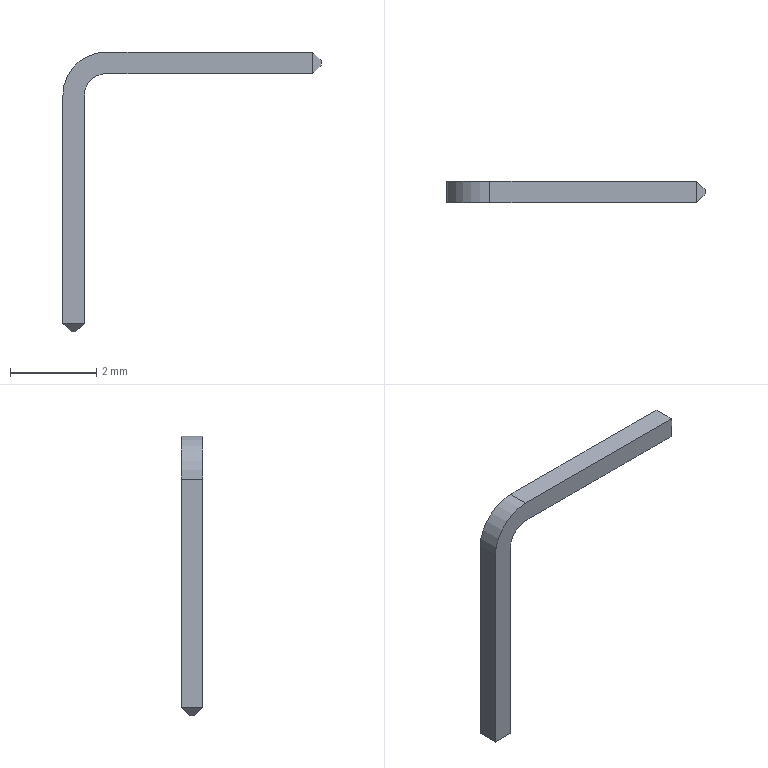Part | STEP file | RJ-USIO-V1_2-220411_57 | 1 solid | 18 faces | box 6 x 0.5 x 6.5 mm | volume 2.861 mm3 | plane 16 | cylinder 2 | commonest cylinder face diameters 1 x1 2 x1
STEP:
#1=CARTESIAN_POINT('',(0.,0.,0.));
#2=DIRECTION('',(0.,0.,1.));
#3=DIRECTION('',(1.,0.,0.));
#4=AXIS2_PLACEMENT_3D('',#1,#2,#3);
#5=CARTESIAN_POINT('',(97.65,59.45,-3.15));
#6=VERTEX_POINT('',#5);
#7=CARTESIAN_POINT('',(97.65,59.35,-3.15));
#8=VERTEX_POINT('',#7);
#9=CARTESIAN_POINT('',(97.65,59.45,-3.15));
#10=DIRECTION('',(0.000000012,-1.,0.));
#11=VECTOR('',#10,1.);
#12=LINE('',#9,#11);
#13=CARTESIAN_POINT('',(97.7,59.4,-3.15));
#14=DIRECTION('',(0.,0.,1.));
#15=DIRECTION('',(0.000000012,-1.,0.));
#16=AXIS2_PLACEMENT_3D('',#13,#14,#15);
#17=PLANE('',#16);
#18=CARTESIAN_POINT('',(-0.05,-0.05));
#19=DIRECTION('',(1.,0.));
#20=VECTOR('',#19,1.);
#21=LINE('',#18,#20);
#22=(GEOMETRIC_REPRESENTATION_CONTEXT(2)PARAMETRIC_REPRESENTATION_CONTEXT()REPRESENTATION_CONTEXT('',''));
#23=DEFINITIONAL_REPRESENTATION('',(#21),#22);
#24=PCURVE('',#17,#23);
#25=CARTESIAN_POINT('',(97.55,59.4,-3.05));
#26=DIRECTION('',(-0.7071,-0.000000008,-0.7071));
#27=DIRECTION('',(-0.7071,-0.000000008,0.7071));
#28=AXIS2_PLACEMENT_3D('',#25,#26,#27);
#29=PLANE('',#28);
#30=CARTESIAN_POINT('',(-0.1414,0.05));
#31=DIRECTION('',(0.,-1.));
#32=VECTOR('',#31,1.);
#33=LINE('',#30,#32);
#34=(GEOMETRIC_REPRESENTATION_CONTEXT(2)PARAMETRIC_REPRESENTATION_CONTEXT()REPRESENTATION_CONTEXT('',''));
#35=DEFINITIONAL_REPRESENTATION('',(#33),#34);
#36=PCURVE('',#29,#35);
#37=SURFACE_CURVE('',#12,(#24,#36),.PCURVE_S1.);
#38=EDGE_CURVE('',#6,#8,#37,.T.);
#39=ORIENTED_EDGE('',*,*,#38,.T.);
#40=CARTESIAN_POINT('',(97.75,59.35,-3.15));
#41=VERTEX_POINT('',#40);
#42=CARTESIAN_POINT('',(97.65,59.35,-3.15));
#43=DIRECTION('',(1.,0.000000012,0.));
#44=VECTOR('',#43,1.);
#45=LINE('',#42,#44);
#46=CARTESIAN_POINT('',(0.05,-0.05));
#47=DIRECTION('',(0.,1.));
#48=VECTOR('',#47,1.);
#49=LINE('',#46,#48);
#50=(GEOMETRIC_REPRESENTATION_CONTEXT(2)PARAMETRIC_REPRESENTATION_CONTEXT()REPRESENTATION_CONTEXT('',''));
#51=DEFINITIONAL_REPRESENTATION('',(#49),#50);
#52=PCURVE('',#17,#51);
#53=CARTESIAN_POINT('',(97.7,59.25,-3.05));
#54=DIRECTION('',(-0.000000008,0.7071,0.7071));
#55=DIRECTION('',(-0.000000008,0.7071,-0.7071));
#56=AXIS2_PLACEMENT_3D('',#53,#54,#55);
#57=PLANE('',#56);
#58=CARTESIAN_POINT('',(0.1414,0.05));
#59=DIRECTION('',(0.,-1.));
#60=VECTOR('',#59,1.);
#61=LINE('',#58,#60);
#62=(GEOMETRIC_REPRESENTATION_CONTEXT(2)PARAMETRIC_REPRESENTATION_CONTEXT()REPRESENTATION_CONTEXT('',''));
#63=DEFINITIONAL_REPRESENTATION('',(#61),#62);
#64=PCURVE('',#57,#63);
#65=SURFACE_CURVE('',#45,(#52,#64),.PCURVE_S1.);
#66=EDGE_CURVE('',#8,#41,#65,.T.);
#67=ORIENTED_EDGE('',*,*,#66,.T.);
#68=CARTESIAN_POINT('',(97.75,59.45,-3.15));
#69=VERTEX_POINT('',#68);
#70=CARTESIAN_POINT('',(97.75,59.45,-3.15));
#71=DIRECTION('',(0.000000012,-1.,0.));
#72=VECTOR('',#71,1.);
#73=LINE('',#70,#72);
#74=CARTESIAN_POINT('',(-0.05,0.05));
#75=DIRECTION('',(1.,0.));
#76=VECTOR('',#75,1.);
#77=LINE('',#74,#76);
#78=(GEOMETRIC_REPRESENTATION_CONTEXT(2)PARAMETRIC_REPRESENTATION_CONTEXT()REPRESENTATION_CONTEXT('',''));
#79=DEFINITIONAL_REPRESENTATION('',(#77),#78);
#80=PCURVE('',#17,#79);
#81=CARTESIAN_POINT('',(97.85,59.4,-3.05));
#82=DIRECTION('',(-0.7071,-0.000000008,0.7071));
#83=DIRECTION('',(-0.7071,-0.000000008,-0.7071));
#84=AXIS2_PLACEMENT_3D('',#81,#82,#83);
#85=PLANE('',#84);
#86=CARTESIAN_POINT('',(0.1414,-0.05));
#87=DIRECTION('',(0.,1.));
#88=VECTOR('',#87,1.);
#89=LINE('',#86,#88);
#90=(GEOMETRIC_REPRESENTATION_CONTEXT(2)PARAMETRIC_REPRESENTATION_CONTEXT()REPRESENTATION_CONTEXT('',''));
#91=DEFINITIONAL_REPRESENTATION('',(#89),#90);
#92=PCURVE('',#85,#91);
#93=SURFACE_CURVE('',#73,(#80,#92),.PCURVE_S1.);
#94=EDGE_CURVE('',#69,#41,#93,.T.);
#95=ORIENTED_EDGE('',*,*,#94,.F.);
#96=CARTESIAN_POINT('',(97.75,59.45,-3.15));
#97=DIRECTION('',(-1.,-0.000000012,0.));
#98=VECTOR('',#97,1.);
#99=LINE('',#96,#98);
#100=CARTESIAN_POINT('',(-0.05,0.05));
#101=DIRECTION('',(0.,-1.));
#102=VECTOR('',#101,1.);
#103=LINE('',#100,#102);
#104=(GEOMETRIC_REPRESENTATION_CONTEXT(2)PARAMETRIC_REPRESENTATION_CONTEXT()REPRESENTATION_CONTEXT('',''));
#105=DEFINITIONAL_REPRESENTATION('',(#103),#104);
#106=PCURVE('',#17,#105);
#107=CARTESIAN_POINT('',(97.7,59.55,-3.05));
#108=DIRECTION('',(0.000000008,-0.7071,0.7071));
#109=DIRECTION('',(0.000000008,-0.7071,-0.7071));
#110=AXIS2_PLACEMENT_3D('',#107,#108,#109);
#111=PLANE('',#110);
#112=CARTESIAN_POINT('',(0.1414,0.05));
#113=DIRECTION('',(0.,-1.));
#114=VECTOR('',#113,1.);
#115=LINE('',#112,#114);
#116=(GEOMETRIC_REPRESENTATION_CONTEXT(2)PARAMETRIC_REPRESENTATION_CONTEXT()REPRESENTATION_CONTEXT('',''));
#117=DEFINITIONAL_REPRESENTATION('',(#115),#116);
#118=PCURVE('',#111,#117);
#119=SURFACE_CURVE('',#99,(#106,#118),.PCURVE_S1.);
#120=EDGE_CURVE('',#69,#6,#119,.T.);
#121=ORIENTED_EDGE('',*,*,#120,.T.);
#122=EDGE_LOOP('',(#39,#67,#95,#121));
#123=FACE_BOUND('',#122,.F.);
#124=ADVANCED_FACE('',(#123),#17,.F.);
#125=ORIENTED_EDGE('',*,*,#38,.F.);
#126=CARTESIAN_POINT('',(97.45,59.65,-2.95));
#127=VERTEX_POINT('',#126);
#128=CARTESIAN_POINT('',(97.65,59.45,-3.15));
#129=DIRECTION('',(-0.5774,0.5774,0.5774));
#130=VECTOR('',#129,1.);
#131=LINE('',#128,#130);
#132=CARTESIAN_POINT('',(-0.1414,0.05));
#133=DIRECTION('',(0.8165,0.5774));
#134=VECTOR('',#133,1.);
#135=LINE('',#132,#134);
#136=(GEOMETRIC_REPRESENTATION_CONTEXT(2)PARAMETRIC_REPRESENTATION_CONTEXT()REPRESENTATION_CONTEXT('',''));
#137=DEFINITIONAL_REPRESENTATION('',(#135),#136);
#138=PCURVE('',#29,#137);
#139=CARTESIAN_POINT('',(0.1414,-0.05));
#140=DIRECTION('',(-0.8165,-0.5774));
#141=VECTOR('',#140,1.);
#142=LINE('',#139,#141);
#143=(GEOMETRIC_REPRESENTATION_CONTEXT(2)PARAMETRIC_REPRESENTATION_CONTEXT()REPRESENTATION_CONTEXT('',''));
#144=DEFINITIONAL_REPRESENTATION('',(#142),#143);
#145=PCURVE('',#111,#144);
#146=SURFACE_CURVE('',#131,(#138,#145),.PCURVE_S1.);
#147=EDGE_CURVE('',#6,#127,#146,.T.);
#148=ORIENTED_EDGE('',*,*,#147,.T.);
#149=CARTESIAN_POINT('',(97.45,59.15,-2.95));
#150=VERTEX_POINT('',#149);
#151=CARTESIAN_POINT('',(97.45,59.15,-2.95));
#152=DIRECTION('',(-0.000000012,1.,0.));
#153=VECTOR('',#152,1.);
#154=LINE('',#151,#153);
#155=CARTESIAN_POINT('',(0.1414,-0.25));
#156=DIRECTION('',(0.,1.));
#157=VECTOR('',#156,1.);
#158=LINE('',#155,#157);
#159=(GEOMETRIC_REPRESENTATION_CONTEXT(2)PARAMETRIC_REPRESENTATION_CONTEXT()REPRESENTATION_CONTEXT('',''));
#160=DEFINITIONAL_REPRESENTATION('',(#158),#159);
#161=PCURVE('',#29,#160);
#162=CARTESIAN_POINT('',(97.45,59.4,-0.3));
#163=DIRECTION('',(-1.,-0.000000012,0.));
#164=DIRECTION('',(0.000000012,-1.,0.));
#165=AXIS2_PLACEMENT_3D('',#162,#163,#164);
#166=PLANE('',#165);
#167=CARTESIAN_POINT('',(0.25,-2.65));
#168=DIRECTION('',(-1.,0.));
#169=VECTOR('',#168,1.);
#170=LINE('',#167,#169);
#171=(GEOMETRIC_REPRESENTATION_CONTEXT(2)PARAMETRIC_REPRESENTATION_CONTEXT()REPRESENTATION_CONTEXT('',''));
#172=DEFINITIONAL_REPRESENTATION('',(#170),#171);
#173=PCURVE('',#166,#172);
#174=SURFACE_CURVE('',#154,(#161,#173),.PCURVE_S1.);
#175=EDGE_CURVE('',#150,#127,#174,.T.);
#176=ORIENTED_EDGE('',*,*,#175,.F.);
#177=CARTESIAN_POINT('',(97.65,59.35,-3.15));
#178=DIRECTION('',(-0.5774,-0.5774,0.5774));
#179=VECTOR('',#178,1.);
#180=LINE('',#177,#179);
#181=CARTESIAN_POINT('',(-0.1414,-0.05));
#182=DIRECTION('',(0.8165,-0.5774));
#183=VECTOR('',#182,1.);
#184=LINE('',#181,#183);
#185=(GEOMETRIC_REPRESENTATION_CONTEXT(2)PARAMETRIC_REPRESENTATION_CONTEXT()REPRESENTATION_CONTEXT('',''));
#186=DEFINITIONAL_REPRESENTATION('',(#184),#185);
#187=PCURVE('',#29,#186);
#188=CARTESIAN_POINT('',(0.1414,0.05));
#189=DIRECTION('',(-0.8165,0.5774));
#190=VECTOR('',#189,1.);
#191=LINE('',#188,#190);
#192=(GEOMETRIC_REPRESENTATION_CONTEXT(2)PARAMETRIC_REPRESENTATION_CONTEXT()REPRESENTATION_CONTEXT('',''));
#193=DEFINITIONAL_REPRESENTATION('',(#191),#192);
#194=PCURVE('',#57,#193);
#195=SURFACE_CURVE('',#180,(#187,#194),.PCURVE_S1.);
#196=EDGE_CURVE('',#8,#150,#195,.T.);
#197=ORIENTED_EDGE('',*,*,#196,.F.);
#198=EDGE_LOOP('',(#125,#148,#176,#197));
#199=FACE_BOUND('',#198,.F.);
#200=ADVANCED_FACE('',(#199),#29,.T.);
#201=ORIENTED_EDGE('',*,*,#120,.F.);
#202=CARTESIAN_POINT('',(97.95,59.65,-2.95));
#203=VERTEX_POINT('',#202);
#204=CARTESIAN_POINT('',(97.95,59.65,-2.95));
#205=DIRECTION('',(-0.5774,-0.5774,-0.5774));
#206=VECTOR('',#205,1.);
#207=LINE('',#204,#206);
#208=CARTESIAN_POINT('',(-0.1414,0.25));
#209=DIRECTION('',(0.8165,-0.5774));
#210=VECTOR('',#209,1.);
#211=LINE('',#208,#210);
#212=(GEOMETRIC_REPRESENTATION_CONTEXT(2)PARAMETRIC_REPRESENTATION_CONTEXT()REPRESENTATION_CONTEXT('',''));
#213=DEFINITIONAL_REPRESENTATION('',(#211),#212);
#214=PCURVE('',#111,#213);
#215=CARTESIAN_POINT('',(-0.1414,-0.25));
#216=DIRECTION('',(0.8165,0.5774));
#217=VECTOR('',#216,1.);
#218=LINE('',#215,#217);
#219=(GEOMETRIC_REPRESENTATION_CONTEXT(2)PARAMETRIC_REPRESENTATION_CONTEXT()REPRESENTATION_CONTEXT('',''));
#220=DEFINITIONAL_REPRESENTATION('',(#218),#219);
#221=PCURVE('',#85,#220);
#222=SURFACE_CURVE('',#207,(#214,#221),.PCURVE_S1.);
#223=EDGE_CURVE('',#203,#69,#222,.T.);
#224=ORIENTED_EDGE('',*,*,#223,.F.);
#225=CARTESIAN_POINT('',(97.45,59.65,-2.95));
#226=DIRECTION('',(1.,0.000000012,0.));
#227=VECTOR('',#226,1.);
#228=LINE('',#225,#227);
#229=CARTESIAN_POINT('',(-0.1414,-0.25));
#230=DIRECTION('',(0.,1.));
#231=VECTOR('',#230,1.);
#232=LINE('',#229,#231);
#233=(GEOMETRIC_REPRESENTATION_CONTEXT(2)PARAMETRIC_REPRESENTATION_CONTEXT()REPRESENTATION_CONTEXT('',''));
#234=DEFINITIONAL_REPRESENTATION('',(#232),#233);
#235=PCURVE('',#111,#234);
#236=CARTESIAN_POINT('',(100.35,59.65,0.2));
#237=DIRECTION('',(-0.000000012,1.,0.));
#238=DIRECTION('',(-1.,-0.000000012,0.));
#239=AXIS2_PLACEMENT_3D('',#236,#237,#238);
#240=PLANE('',#239);
#241=CARTESIAN_POINT('',(2.9,-3.15));
#242=DIRECTION('',(-1.,0.));
#243=VECTOR('',#242,1.);
#244=LINE('',#241,#243);
#245=(GEOMETRIC_REPRESENTATION_CONTEXT(2)PARAMETRIC_REPRESENTATION_CONTEXT()REPRESENTATION_CONTEXT('',''));
#246=DEFINITIONAL_REPRESENTATION('',(#244),#245);
#247=PCURVE('',#240,#246);
#248=SURFACE_CURVE('',#228,(#235,#247),.PCURVE_S1.);
#249=EDGE_CURVE('',#127,#203,#248,.T.);
#250=ORIENTED_EDGE('',*,*,#249,.F.);
#251=ORIENTED_EDGE('',*,*,#147,.F.);
#252=EDGE_LOOP('',(#201,#224,#250,#251));
#253=FACE_BOUND('',#252,.F.);
#254=ADVANCED_FACE('',(#253),#111,.F.);
#255=ORIENTED_EDGE('',*,*,#94,.T.);
#256=CARTESIAN_POINT('',(97.95,59.15,-2.95));
#257=VERTEX_POINT('',#256);
#258=CARTESIAN_POINT('',(97.95,59.15,-2.95));
#259=DIRECTION('',(-0.5774,0.5774,-0.5774));
#260=VECTOR('',#259,1.);
#261=LINE('',#258,#260);
#262=CARTESIAN_POINT('',(-0.1414,0.25));
#263=DIRECTION('',(0.8165,-0.5774));
#264=VECTOR('',#263,1.);
#265=LINE('',#262,#264);
#266=(GEOMETRIC_REPRESENTATION_CONTEXT(2)PARAMETRIC_REPRESENTATION_CONTEXT()REPRESENTATION_CONTEXT('',''));
#267=DEFINITIONAL_REPRESENTATION('',(#265),#266);
#268=PCURVE('',#85,#267);
#269=CARTESIAN_POINT('',(-0.1414,-0.25));
#270=DIRECTION('',(0.8165,0.5774));
#271=VECTOR('',#270,1.);
#272=LINE('',#269,#271);
#273=(GEOMETRIC_REPRESENTATION_CONTEXT(2)PARAMETRIC_REPRESENTATION_CONTEXT()REPRESENTATION_CONTEXT('',''));
#274=DEFINITIONAL_REPRESENTATION('',(#272),#273);
#275=PCURVE('',#57,#274);
#276=SURFACE_CURVE('',#261,(#268,#275),.PCURVE_S1.);
#277=EDGE_CURVE('',#257,#41,#276,.T.);
#278=ORIENTED_EDGE('',*,*,#277,.F.);
#279=CARTESIAN_POINT('',(97.95,59.65,-2.95));
#280=DIRECTION('',(0.000000012,-1.,0.));
#281=VECTOR('',#280,1.);
#282=LINE('',#279,#281);
#283=CARTESIAN_POINT('',(-0.1414,-0.25));
#284=DIRECTION('',(0.,1.));
#285=VECTOR('',#284,1.);
#286=LINE('',#283,#285);
#287=(GEOMETRIC_REPRESENTATION_CONTEXT(2)PARAMETRIC_REPRESENTATION_CONTEXT()REPRESENTATION_CONTEXT('',''));
#288=DEFINITIONAL_REPRESENTATION('',(#286),#287);
#289=PCURVE('',#85,#288);
#290=CARTESIAN_POINT('',(97.95,59.4,-0.3));
#291=DIRECTION('',(-1.,-0.000000012,0.));
#292=DIRECTION('',(-0.000000012,1.,0.));
#293=AXIS2_PLACEMENT_3D('',#290,#291,#292);
#294=PLANE('',#293);
#295=CARTESIAN_POINT('',(0.25,2.65));
#296=DIRECTION('',(-1.,0.));
#297=VECTOR('',#296,1.);
#298=LINE('',#295,#297);
#299=(GEOMETRIC_REPRESENTATION_CONTEXT(2)PARAMETRIC_REPRESENTATION_CONTEXT()REPRESENTATION_CONTEXT('',''));
#300=DEFINITIONAL_REPRESENTATION('',(#298),#299);
#301=PCURVE('',#294,#300);
#302=SURFACE_CURVE('',#282,(#289,#301),.PCURVE_S1.);
#303=EDGE_CURVE('',#203,#257,#302,.T.);
#304=ORIENTED_EDGE('',*,*,#303,.F.);
#305=ORIENTED_EDGE('',*,*,#223,.T.);
#306=EDGE_LOOP('',(#255,#278,#304,#305));
#307=FACE_BOUND('',#306,.F.);
#308=ADVANCED_FACE('',(#307),#85,.F.);
#309=ORIENTED_EDGE('',*,*,#66,.F.);
#310=ORIENTED_EDGE('',*,*,#196,.T.);
#311=CARTESIAN_POINT('',(97.45,59.15,-2.95));
#312=DIRECTION('',(1.,0.000000012,0.));
#313=VECTOR('',#312,1.);
#314=LINE('',#311,#313);
#315=CARTESIAN_POINT('',(-0.1414,0.25));
#316=DIRECTION('',(0.,-1.));
#317=VECTOR('',#316,1.);
#318=LINE('',#315,#317);
#319=(GEOMETRIC_REPRESENTATION_CONTEXT(2)PARAMETRIC_REPRESENTATION_CONTEXT()REPRESENTATION_CONTEXT('',''));
#320=DEFINITIONAL_REPRESENTATION('',(#318),#319);
#321=PCURVE('',#57,#320);
#322=CARTESIAN_POINT('',(100.35,59.15,0.2));
#323=DIRECTION('',(-0.000000012,1.,0.));
#324=DIRECTION('',(-1.,-0.000000012,0.));
#325=AXIS2_PLACEMENT_3D('',#322,#323,#324);
#326=PLANE('',#325);
#327=CARTESIAN_POINT('',(2.9,-3.15));
#328=DIRECTION('',(-1.,0.));
#329=VECTOR('',#328,1.);
#330=LINE('',#327,#329);
#331=(GEOMETRIC_REPRESENTATION_CONTEXT(2)PARAMETRIC_REPRESENTATION_CONTEXT()REPRESENTATION_CONTEXT('',''));
#332=DEFINITIONAL_REPRESENTATION('',(#330),#331);
#333=PCURVE('',#326,#332);
#334=SURFACE_CURVE('',#314,(#321,#333),.PCURVE_S1.);
#335=EDGE_CURVE('',#150,#257,#334,.T.);
#336=ORIENTED_EDGE('',*,*,#335,.T.);
#337=ORIENTED_EDGE('',*,*,#277,.T.);
#338=EDGE_LOOP('',(#309,#310,#336,#337));
#339=FACE_BOUND('',#338,.F.);
#340=ADVANCED_FACE('',(#339),#57,.F.);
#341=CARTESIAN_POINT('',(97.95,59.15,2.35));
#342=VERTEX_POINT('',#341);
#343=CARTESIAN_POINT('',(98.45,59.15,2.85));
#344=VERTEX_POINT('',#343);
#345=CARTESIAN_POINT('',(98.45,59.15,2.35));
#346=DIRECTION('',(-0.000000012,1.,0.));
#347=DIRECTION('',(-1.,-0.000000012,0.000000014));
#348=AXIS2_PLACEMENT_3D('',#345,#346,#347);
#349=CIRCLE('',#348,0.5);
#350=CARTESIAN_POINT('',(1.9,2.15));
#351=DIRECTION('',(1.,0.000000014));
#352=AXIS2_PLACEMENT_2D('',#350,#351);
#353=CIRCLE('',#352,0.5);
#354=(GEOMETRIC_REPRESENTATION_CONTEXT(2)PARAMETRIC_REPRESENTATION_CONTEXT()REPRESENTATION_CONTEXT('',''));
#355=DEFINITIONAL_REPRESENTATION('',(#353),#354);
#356=PCURVE('',#326,#355);
#357=CARTESIAN_POINT('',(98.45,59.65,2.35));
#358=DIRECTION('',(0.000000012,-1.,0.));
#359=DIRECTION('',(-1.,-0.000000012,0.));
#360=AXIS2_PLACEMENT_3D('',#357,#358,#359);
#361=CYLINDRICAL_SURFACE('',#360,0.5);
#362=CARTESIAN_POINT('',(6.283,0.5));
#363=DIRECTION('',(-1.,0.));
#364=VECTOR('',#363,1.);
#365=LINE('',#362,#364);
#366=(GEOMETRIC_REPRESENTATION_CONTEXT(2)PARAMETRIC_REPRESENTATION_CONTEXT()REPRESENTATION_CONTEXT('',''));
#367=DEFINITIONAL_REPRESENTATION('',(#365),#366);
#368=PCURVE('',#361,#367);
#369=SURFACE_CURVE('',#349,(#356,#368),.PCURVE_S1.);
#370=EDGE_CURVE('',#342,#344,#369,.T.);
#371=ORIENTED_EDGE('',*,*,#370,.F.);
#372=CARTESIAN_POINT('',(97.95,59.15,2.35));
#373=DIRECTION('',(0.,0.,-1.));
#374=VECTOR('',#373,1.);
#375=LINE('',#372,#374);
#376=CARTESIAN_POINT('',(2.4,2.15));
#377=DIRECTION('',(0.,-1.));
#378=VECTOR('',#377,1.);
#379=LINE('',#376,#378);
#380=(GEOMETRIC_REPRESENTATION_CONTEXT(2)PARAMETRIC_REPRESENTATION_CONTEXT()REPRESENTATION_CONTEXT('',''));
#381=DEFINITIONAL_REPRESENTATION('',(#379),#380);
#382=PCURVE('',#326,#381);
#383=CARTESIAN_POINT('',(-0.25,-2.65));
#384=DIRECTION('',(0.,1.));
#385=VECTOR('',#384,1.);
#386=LINE('',#383,#385);
#387=(GEOMETRIC_REPRESENTATION_CONTEXT(2)PARAMETRIC_REPRESENTATION_CONTEXT()REPRESENTATION_CONTEXT('',''));
#388=DEFINITIONAL_REPRESENTATION('',(#386),#387);
#389=PCURVE('',#294,#388);
#390=SURFACE_CURVE('',#375,(#382,#389),.PCURVE_S1.);
#391=EDGE_CURVE('',#342,#257,#390,.T.);
#392=ORIENTED_EDGE('',*,*,#391,.T.);
#393=ORIENTED_EDGE('',*,*,#335,.F.);
#394=CARTESIAN_POINT('',(97.45,59.15,2.35));
#395=VERTEX_POINT('',#394);
#396=CARTESIAN_POINT('',(97.45,59.15,-2.95));
#397=DIRECTION('',(0.,0.,1.));
#398=VECTOR('',#397,1.);
#399=LINE('',#396,#398);
#400=CARTESIAN_POINT('',(2.9,-3.15));
#401=DIRECTION('',(0.,1.));
#402=VECTOR('',#401,1.);
#403=LINE('',#400,#402);
#404=(GEOMETRIC_REPRESENTATION_CONTEXT(2)PARAMETRIC_REPRESENTATION_CONTEXT()REPRESENTATION_CONTEXT('',''));
#405=DEFINITIONAL_REPRESENTATION('',(#403),#404);
#406=PCURVE('',#326,#405);
#407=CARTESIAN_POINT('',(0.25,-2.65));
#408=DIRECTION('',(0.,1.));
#409=VECTOR('',#408,1.);
#410=LINE('',#407,#409);
#411=(GEOMETRIC_REPRESENTATION_CONTEXT(2)PARAMETRIC_REPRESENTATION_CONTEXT()REPRESENTATION_CONTEXT('',''));
#412=DEFINITIONAL_REPRESENTATION('',(#410),#411);
#413=PCURVE('',#166,#412);
#414=SURFACE_CURVE('',#399,(#406,#413),.PCURVE_S1.);
#415=EDGE_CURVE('',#150,#395,#414,.T.);
#416=ORIENTED_EDGE('',*,*,#415,.T.);
#417=CARTESIAN_POINT('',(98.45,59.15,3.35));
#418=VERTEX_POINT('',#417);
#419=CARTESIAN_POINT('',(98.45,59.15,2.35));
#420=DIRECTION('',(0.000000012,-1.,0.));
#421=DIRECTION('',(-0.000000001,0.,1.));
#422=AXIS2_PLACEMENT_3D('',#419,#420,#421);
#423=CIRCLE('',#422,1.);
#424=CARTESIAN_POINT('',(1.9,3.15));
#425=CARTESIAN_POINT('',(3.632,3.15));
#426=CARTESIAN_POINT('',(2.766,1.65));
#427=CARTESIAN_POINT('',(1.9,0.15));
#428=CARTESIAN_POINT('',(1.034,1.65));
#429=CARTESIAN_POINT('',(0.1679,3.15));
#430=CARTESIAN_POINT('',(1.9,3.15));
#431=(BOUNDED_CURVE()B_SPLINE_CURVE(2,(#424,#425,#426,#427,#428,#429,#430),.UNSPECIFIED.,.T.,.F.)B_SPLINE_CURVE_WITH_KNOTS((1,2,2,2,2,1),(-2.094,0.,2.094,4.189,6.283,8.378),.UNSPECIFIED.)CURVE()GEOMETRIC_REPRESENTATION_ITEM()RATIONAL_B_SPLINE_CURVE((1.,0.5,1.,0.5,1.,0.5,1.))REPRESENTATION_ITEM(''));
#432=(GEOMETRIC_REPRESENTATION_CONTEXT(2)PARAMETRIC_REPRESENTATION_CONTEXT()REPRESENTATION_CONTEXT('',''));
#433=DEFINITIONAL_REPRESENTATION('',(#431),#432);
#434=PCURVE('',#326,#433);
#435=CARTESIAN_POINT('',(98.45,59.65,2.35));
#436=DIRECTION('',(0.000000012,-1.,0.));
#437=DIRECTION('',(-1.,-0.000000012,0.));
#438=AXIS2_PLACEMENT_3D('',#435,#436,#437);
#439=CYLINDRICAL_SURFACE('',#438,1.);
#440=CARTESIAN_POINT('',(4.712,0.5));
#441=DIRECTION('',(1.,0.));
#442=VECTOR('',#441,1.);
#443=LINE('',#440,#442);
#444=(GEOMETRIC_REPRESENTATION_CONTEXT(2)PARAMETRIC_REPRESENTATION_CONTEXT()REPRESENTATION_CONTEXT('',''));
#445=DEFINITIONAL_REPRESENTATION('',(#443),#444);
#446=PCURVE('',#439,#445);
#447=SURFACE_CURVE('',#423,(#434,#446),.PCURVE_S1.);
#448=EDGE_CURVE('',#418,#395,#447,.T.);
#449=ORIENTED_EDGE('',*,*,#448,.F.);
#450=CARTESIAN_POINT('',(103.25,59.15,3.35));
#451=VERTEX_POINT('',#450);
#452=CARTESIAN_POINT('',(98.45,59.15,3.35));
#453=DIRECTION('',(1.,0.000000012,0.));
#454=VECTOR('',#453,1.);
#455=LINE('',#452,#454);
#456=CARTESIAN_POINT('',(1.9,3.15));
#457=DIRECTION('',(-1.,0.));
#458=VECTOR('',#457,1.);
#459=LINE('',#456,#458);
#460=(GEOMETRIC_REPRESENTATION_CONTEXT(2)PARAMETRIC_REPRESENTATION_CONTEXT()REPRESENTATION_CONTEXT('',''));
#461=DEFINITIONAL_REPRESENTATION('',(#459),#460);
#462=PCURVE('',#326,#461);
#463=CARTESIAN_POINT('',(100.85,59.4,3.35));
#464=DIRECTION('',(0.,0.,1.));
#465=DIRECTION('',(-0.000000012,1.,0.));
#466=AXIS2_PLACEMENT_3D('',#463,#464,#465);
#467=PLANE('',#466);
#468=CARTESIAN_POINT('',(-0.25,2.4));
#469=DIRECTION('',(0.,-1.));
#470=VECTOR('',#469,1.);
#471=LINE('',#468,#470);
#472=(GEOMETRIC_REPRESENTATION_CONTEXT(2)PARAMETRIC_REPRESENTATION_CONTEXT()REPRESENTATION_CONTEXT('',''));
#473=DEFINITIONAL_REPRESENTATION('',(#471),#472);
#474=PCURVE('',#467,#473);
#475=SURFACE_CURVE('',#455,(#462,#474),.PCURVE_S1.);
#476=EDGE_CURVE('',#418,#451,#475,.T.);
#477=ORIENTED_EDGE('',*,*,#476,.T.);
#478=CARTESIAN_POINT('',(103.25,59.15,2.85));
#479=VERTEX_POINT('',#478);
#480=CARTESIAN_POINT('',(103.25,59.15,2.85));
#481=DIRECTION('',(0.,0.,1.));
#482=VECTOR('',#481,1.);
#483=LINE('',#480,#482);
#484=CARTESIAN_POINT('',(-2.9,2.65));
#485=DIRECTION('',(0.,1.));
#486=VECTOR('',#485,1.);
#487=LINE('',#484,#486);
#488=(GEOMETRIC_REPRESENTATION_CONTEXT(2)PARAMETRIC_REPRESENTATION_CONTEXT()REPRESENTATION_CONTEXT('',''));
#489=DEFINITIONAL_REPRESENTATION('',(#487),#488);
#490=PCURVE('',#326,#489);
#491=CARTESIAN_POINT('',(103.35,59.25,3.1));
#492=DIRECTION('',(-0.7071,0.7071,0.));
#493=DIRECTION('',(-0.7071,-0.7071,0.));
#494=AXIS2_PLACEMENT_3D('',#491,#492,#493);
#495=PLANE('',#494);
#496=CARTESIAN_POINT('',(0.1414,-0.25));
#497=DIRECTION('',(0.,1.));
#498=VECTOR('',#497,1.);
#499=LINE('',#496,#498);
#500=(GEOMETRIC_REPRESENTATION_CONTEXT(2)PARAMETRIC_REPRESENTATION_CONTEXT()REPRESENTATION_CONTEXT('',''));
#501=DEFINITIONAL_REPRESENTATION('',(#499),#500);
#502=PCURVE('',#495,#501);
#503=SURFACE_CURVE('',#483,(#490,#502),.PCURVE_S1.);
#504=EDGE_CURVE('',#479,#451,#503,.T.);
#505=ORIENTED_EDGE('',*,*,#504,.F.);
#506=CARTESIAN_POINT('',(103.25,59.15,2.85));
#507=DIRECTION('',(-1.,-0.000000012,0.));
#508=VECTOR('',#507,1.);
#509=LINE('',#506,#508);
#510=CARTESIAN_POINT('',(-2.9,2.65));
#511=DIRECTION('',(1.,0.));
#512=VECTOR('',#511,1.);
#513=LINE('',#510,#512);
#514=(GEOMETRIC_REPRESENTATION_CONTEXT(2)PARAMETRIC_REPRESENTATION_CONTEXT()REPRESENTATION_CONTEXT('',''));
#515=DEFINITIONAL_REPRESENTATION('',(#513),#514);
#516=PCURVE('',#326,#515);
#517=CARTESIAN_POINT('',(100.85,59.4,2.85));
#518=DIRECTION('',(0.,0.,1.));
#519=DIRECTION('',(-1.,-0.000000012,0.));
#520=AXIS2_PLACEMENT_3D('',#517,#518,#519);
#521=PLANE('',#520);
#522=CARTESIAN_POINT('',(-2.4,0.25));
#523=DIRECTION('',(1.,0.));
#524=VECTOR('',#523,1.);
#525=LINE('',#522,#524);
#526=(GEOMETRIC_REPRESENTATION_CONTEXT(2)PARAMETRIC_REPRESENTATION_CONTEXT()REPRESENTATION_CONTEXT('',''));
#527=DEFINITIONAL_REPRESENTATION('',(#525),#526);
#528=PCURVE('',#521,#527);
#529=SURFACE_CURVE('',#509,(#516,#528),.PCURVE_S1.);
#530=EDGE_CURVE('',#479,#344,#529,.T.);
#531=ORIENTED_EDGE('',*,*,#530,.T.);
#532=EDGE_LOOP('',(#371,#392,#393,#416,#449,#477,#505,#531));
#533=FACE_BOUND('',#532,.F.);
#534=ADVANCED_FACE('',(#533),#326,.F.);
#535=CARTESIAN_POINT('',(97.95,59.65,2.35));
#536=VERTEX_POINT('',#535);
#537=CARTESIAN_POINT('',(97.95,59.15,2.35));
#538=DIRECTION('',(-0.000000012,1.,0.));
#539=VECTOR('',#538,1.);
#540=LINE('',#537,#539);
#541=CARTESIAN_POINT('',(6.283,0.5));
#542=DIRECTION('',(0.,-1.));
#543=VECTOR('',#542,1.);
#544=LINE('',#541,#543);
#545=(GEOMETRIC_REPRESENTATION_CONTEXT(2)PARAMETRIC_REPRESENTATION_CONTEXT()REPRESENTATION_CONTEXT('',''));
#546=DEFINITIONAL_REPRESENTATION('',(#544),#545);
#547=PCURVE('',#361,#546);
#548=CARTESIAN_POINT('',(-0.25,-2.65));
#549=DIRECTION('',(1.,0.));
#550=VECTOR('',#549,1.);
#551=LINE('',#548,#550);
#552=(GEOMETRIC_REPRESENTATION_CONTEXT(2)PARAMETRIC_REPRESENTATION_CONTEXT()REPRESENTATION_CONTEXT('',''));
#553=DEFINITIONAL_REPRESENTATION('',(#551),#552);
#554=PCURVE('',#294,#553);
#555=SURFACE_CURVE('',#540,(#547,#554),.PCURVE_S1.);
#556=EDGE_CURVE('',#342,#536,#555,.T.);
#557=ORIENTED_EDGE('',*,*,#556,.F.);
#558=ORIENTED_EDGE('',*,*,#370,.T.);
#559=CARTESIAN_POINT('',(98.45,59.65,2.85));
#560=VERTEX_POINT('',#559);
#561=CARTESIAN_POINT('',(98.45,59.65,2.85));
#562=DIRECTION('',(0.000000012,-1.,0.));
#563=VECTOR('',#562,1.);
#564=LINE('',#561,#563);
#565=CARTESIAN_POINT('',(4.712,0.));
#566=DIRECTION('',(0.,1.));
#567=VECTOR('',#566,1.);
#568=LINE('',#565,#567);
#569=(GEOMETRIC_REPRESENTATION_CONTEXT(2)PARAMETRIC_REPRESENTATION_CONTEXT()REPRESENTATION_CONTEXT('',''));
#570=DEFINITIONAL_REPRESENTATION('',(#568),#569);
#571=PCURVE('',#361,#570);
#572=CARTESIAN_POINT('',(2.4,-0.25));
#573=DIRECTION('',(0.,1.));
#574=VECTOR('',#573,1.);
#575=LINE('',#572,#574);
#576=(GEOMETRIC_REPRESENTATION_CONTEXT(2)PARAMETRIC_REPRESENTATION_CONTEXT()REPRESENTATION_CONTEXT('',''));
#577=DEFINITIONAL_REPRESENTATION('',(#575),#576);
#578=PCURVE('',#521,#577);
#579=SURFACE_CURVE('',#564,(#571,#578),.PCURVE_S1.);
#580=EDGE_CURVE('',#560,#344,#579,.T.);
#581=ORIENTED_EDGE('',*,*,#580,.F.);
#582=CARTESIAN_POINT('',(98.45,59.65,2.35));
#583=DIRECTION('',(0.000000012,-1.,0.));
#584=DIRECTION('',(0.000000015,0.,1.));
#585=AXIS2_PLACEMENT_3D('',#582,#583,#584);
#586=CIRCLE('',#585,0.5);
#587=CARTESIAN_POINT('',(4.712,0.));
#588=DIRECTION('',(1.,0.));
#589=VECTOR('',#588,1.);
#590=LINE('',#587,#589);
#591=(GEOMETRIC_REPRESENTATION_CONTEXT(2)PARAMETRIC_REPRESENTATION_CONTEXT()REPRESENTATION_CONTEXT('',''));
#592=DEFINITIONAL_REPRESENTATION('',(#590),#591);
#593=PCURVE('',#361,#592);
#594=CARTESIAN_POINT('',(1.9,2.65));
#595=CARTESIAN_POINT('',(2.766,2.65));
#596=CARTESIAN_POINT('',(2.333,1.9));
#597=CARTESIAN_POINT('',(1.9,1.15));
#598=CARTESIAN_POINT('',(1.467,1.9));
#599=CARTESIAN_POINT('',(1.034,2.65));
#600=CARTESIAN_POINT('',(1.9,2.65));
#601=(BOUNDED_CURVE()B_SPLINE_CURVE(2,(#594,#595,#596,#597,#598,#599,#600),.UNSPECIFIED.,.T.,.F.)B_SPLINE_CURVE_WITH_KNOTS((1,2,2,2,2,1),(-2.094,0.,2.094,4.189,6.283,8.378),.UNSPECIFIED.)CURVE()GEOMETRIC_REPRESENTATION_ITEM()RATIONAL_B_SPLINE_CURVE((1.,0.5,1.,0.5,1.,0.5,1.))REPRESENTATION_ITEM(''));
#602=(GEOMETRIC_REPRESENTATION_CONTEXT(2)PARAMETRIC_REPRESENTATION_CONTEXT()REPRESENTATION_CONTEXT('',''));
#603=DEFINITIONAL_REPRESENTATION('',(#601),#602);
#604=PCURVE('',#240,#603);
#605=SURFACE_CURVE('',#586,(#593,#604),.PCURVE_S1.);
#606=EDGE_CURVE('',#560,#536,#605,.T.);
#607=ORIENTED_EDGE('',*,*,#606,.T.);
#608=EDGE_LOOP('',(#557,#558,#581,#607));
#609=FACE_BOUND('',#608,.F.);
#610=ADVANCED_FACE('',(#609),#361,.F.);
#611=ORIENTED_EDGE('',*,*,#303,.T.);
#612=ORIENTED_EDGE('',*,*,#391,.F.);
#613=ORIENTED_EDGE('',*,*,#556,.T.);
#614=CARTESIAN_POINT('',(97.95,59.65,-2.95));
#615=DIRECTION('',(0.,0.,1.));
#616=VECTOR('',#615,1.);
#617=LINE('',#614,#616);
#618=CARTESIAN_POINT('',(0.25,2.65));
#619=DIRECTION('',(0.,-1.));
#620=VECTOR('',#619,1.);
#621=LINE('',#618,#620);
#622=(GEOMETRIC_REPRESENTATION_CONTEXT(2)PARAMETRIC_REPRESENTATION_CONTEXT()REPRESENTATION_CONTEXT('',''));
#623=DEFINITIONAL_REPRESENTATION('',(#621),#622);
#624=PCURVE('',#294,#623);
#625=CARTESIAN_POINT('',(2.4,-3.15));
#626=DIRECTION('',(0.,1.));
#627=VECTOR('',#626,1.);
#628=LINE('',#625,#627);
#629=(GEOMETRIC_REPRESENTATION_CONTEXT(2)PARAMETRIC_REPRESENTATION_CONTEXT()REPRESENTATION_CONTEXT('',''));
#630=DEFINITIONAL_REPRESENTATION('',(#628),#629);
#631=PCURVE('',#240,#630);
#632=SURFACE_CURVE('',#617,(#624,#631),.PCURVE_S1.);
#633=EDGE_CURVE('',#203,#536,#632,.T.);
#634=ORIENTED_EDGE('',*,*,#633,.F.);
#635=EDGE_LOOP('',(#611,#612,#613,#634));
#636=FACE_BOUND('',#635,.F.);
#637=ADVANCED_FACE('',(#636),#294,.F.);
#638=CARTESIAN_POINT('',(103.25,59.65,2.85));
#639=VERTEX_POINT('',#638);
#640=CARTESIAN_POINT('',(103.25,59.65,3.35));
#641=VERTEX_POINT('',#640);
#642=CARTESIAN_POINT('',(103.25,59.65,2.85));
#643=DIRECTION('',(0.,0.,1.));
#644=VECTOR('',#643,1.);
#645=LINE('',#642,#644);
#646=CARTESIAN_POINT('',(-2.9,2.65));
#647=DIRECTION('',(0.,1.));
#648=VECTOR('',#647,1.);
#649=LINE('',#646,#648);
#650=(GEOMETRIC_REPRESENTATION_CONTEXT(2)PARAMETRIC_REPRESENTATION_CONTEXT()REPRESENTATION_CONTEXT('',''));
#651=DEFINITIONAL_REPRESENTATION('',(#649),#650);
#652=PCURVE('',#240,#651);
#653=CARTESIAN_POINT('',(103.35,59.55,3.1));
#654=DIRECTION('',(-0.7071,-0.7071,0.));
#655=DIRECTION('',(-0.7071,0.7071,0.));
#656=AXIS2_PLACEMENT_3D('',#653,#654,#655);
#657=PLANE('',#656);
#658=CARTESIAN_POINT('',(0.1414,0.25));
#659=DIRECTION('',(0.,-1.));
#660=VECTOR('',#659,1.);
#661=LINE('',#658,#660);
#662=(GEOMETRIC_REPRESENTATION_CONTEXT(2)PARAMETRIC_REPRESENTATION_CONTEXT()REPRESENTATION_CONTEXT('',''));
#663=DEFINITIONAL_REPRESENTATION('',(#661),#662);
#664=PCURVE('',#657,#663);
#665=SURFACE_CURVE('',#645,(#652,#664),.PCURVE_S1.);
#666=EDGE_CURVE('',#639,#641,#665,.T.);
#667=ORIENTED_EDGE('',*,*,#666,.T.);
#668=CARTESIAN_POINT('',(98.45,59.65,3.35));
#669=VERTEX_POINT('',#668);
#670=CARTESIAN_POINT('',(103.25,59.65,3.35));
#671=DIRECTION('',(-1.,-0.000000012,0.));
#672=VECTOR('',#671,1.);
#673=LINE('',#670,#672);
#674=CARTESIAN_POINT('',(-2.9,3.15));
#675=DIRECTION('',(1.,0.));
#676=VECTOR('',#675,1.);
#677=LINE('',#674,#676);
#678=(GEOMETRIC_REPRESENTATION_CONTEXT(2)PARAMETRIC_REPRESENTATION_CONTEXT()REPRESENTATION_CONTEXT('',''));
#679=DEFINITIONAL_REPRESENTATION('',(#677),#678);
#680=PCURVE('',#240,#679);
#681=CARTESIAN_POINT('',(0.25,-2.4));
#682=DIRECTION('',(0.,1.));
#683=VECTOR('',#682,1.);
#684=LINE('',#681,#683);
#685=(GEOMETRIC_REPRESENTATION_CONTEXT(2)PARAMETRIC_REPRESENTATION_CONTEXT()REPRESENTATION_CONTEXT('',''));
#686=DEFINITIONAL_REPRESENTATION('',(#684),#685);
#687=PCURVE('',#467,#686);
#688=SURFACE_CURVE('',#673,(#680,#687),.PCURVE_S1.);
#689=EDGE_CURVE('',#641,#669,#688,.T.);
#690=ORIENTED_EDGE('',*,*,#689,.T.);
#691=CARTESIAN_POINT('',(97.45,59.65,2.35));
#692=VERTEX_POINT('',#691);
#693=CARTESIAN_POINT('',(98.45,59.65,2.35));
#694=DIRECTION('',(-0.000000012,1.,0.));
#695=DIRECTION('',(-1.,-0.000000012,-0.000000001));
#696=AXIS2_PLACEMENT_3D('',#693,#694,#695);
#697=CIRCLE('',#696,1.);
#698=CARTESIAN_POINT('',(1.9,2.15));
#699=DIRECTION('',(1.,-0.000000001));
#700=AXIS2_PLACEMENT_2D('',#698,#699);
#701=CIRCLE('',#700,1.);
#702=(GEOMETRIC_REPRESENTATION_CONTEXT(2)PARAMETRIC_REPRESENTATION_CONTEXT()REPRESENTATION_CONTEXT('',''));
#703=DEFINITIONAL_REPRESENTATION('',(#701),#702);
#704=PCURVE('',#240,#703);
#705=CARTESIAN_POINT('',(6.283,0.));
#706=DIRECTION('',(-1.,0.));
#707=VECTOR('',#706,1.);
#708=LINE('',#705,#707);
#709=(GEOMETRIC_REPRESENTATION_CONTEXT(2)PARAMETRIC_REPRESENTATION_CONTEXT()REPRESENTATION_CONTEXT('',''));
#710=DEFINITIONAL_REPRESENTATION('',(#708),#709);
#711=PCURVE('',#439,#710);
#712=SURFACE_CURVE('',#697,(#704,#711),.PCURVE_S1.);
#713=EDGE_CURVE('',#692,#669,#712,.T.);
#714=ORIENTED_EDGE('',*,*,#713,.F.);
#715=CARTESIAN_POINT('',(97.45,59.65,2.35));
#716=DIRECTION('',(0.,0.,-1.));
#717=VECTOR('',#716,1.);
#718=LINE('',#715,#717);
#719=CARTESIAN_POINT('',(2.9,2.15));
#720=DIRECTION('',(0.,-1.));
#721=VECTOR('',#720,1.);
#722=LINE('',#719,#721);
#723=(GEOMETRIC_REPRESENTATION_CONTEXT(2)PARAMETRIC_REPRESENTATION_CONTEXT()REPRESENTATION_CONTEXT('',''));
#724=DEFINITIONAL_REPRESENTATION('',(#722),#723);
#725=PCURVE('',#240,#724);
#726=CARTESIAN_POINT('',(-0.25,2.65));
#727=DIRECTION('',(0.,-1.));
#728=VECTOR('',#727,1.);
#729=LINE('',#726,#728);
#730=(GEOMETRIC_REPRESENTATION_CONTEXT(2)PARAMETRIC_REPRESENTATION_CONTEXT()REPRESENTATION_CONTEXT('',''));
#731=DEFINITIONAL_REPRESENTATION('',(#729),#730);
#732=PCURVE('',#166,#731);
#733=SURFACE_CURVE('',#718,(#725,#732),.PCURVE_S1.);
#734=EDGE_CURVE('',#692,#127,#733,.T.);
#735=ORIENTED_EDGE('',*,*,#734,.T.);
#736=ORIENTED_EDGE('',*,*,#249,.T.);
#737=ORIENTED_EDGE('',*,*,#633,.T.);
#738=ORIENTED_EDGE('',*,*,#606,.F.);
#739=CARTESIAN_POINT('',(98.45,59.65,2.85));
#740=DIRECTION('',(1.,0.000000012,0.));
#741=VECTOR('',#740,1.);
#742=LINE('',#739,#741);
#743=CARTESIAN_POINT('',(1.9,2.65));
#744=DIRECTION('',(-1.,0.));
#745=VECTOR('',#744,1.);
#746=LINE('',#743,#745);
#747=(GEOMETRIC_REPRESENTATION_CONTEXT(2)PARAMETRIC_REPRESENTATION_CONTEXT()REPRESENTATION_CONTEXT('',''));
#748=DEFINITIONAL_REPRESENTATION('',(#746),#747);
#749=PCURVE('',#240,#748);
#750=CARTESIAN_POINT('',(2.4,-0.25));
#751=DIRECTION('',(-1.,0.));
#752=VECTOR('',#751,1.);
#753=LINE('',#750,#752);
#754=(GEOMETRIC_REPRESENTATION_CONTEXT(2)PARAMETRIC_REPRESENTATION_CONTEXT()REPRESENTATION_CONTEXT('',''));
#755=DEFINITIONAL_REPRESENTATION('',(#753),#754);
#756=PCURVE('',#521,#755);
#757=SURFACE_CURVE('',#742,(#749,#756),.PCURVE_S1.);
#758=EDGE_CURVE('',#560,#639,#757,.T.);
#759=ORIENTED_EDGE('',*,*,#758,.T.);
#760=EDGE_LOOP('',(#667,#690,#714,#735,#736,#737,#738,#759));
#761=FACE_BOUND('',#760,.F.);
#762=ADVANCED_FACE('',(#761),#240,.T.);
#763=ORIENTED_EDGE('',*,*,#666,.F.);
#764=CARTESIAN_POINT('',(103.45,59.45,3.05));
#765=VERTEX_POINT('',#764);
#766=CARTESIAN_POINT('',(103.45,59.45,3.05));
#767=DIRECTION('',(-0.5774,0.5774,-0.5774));
#768=VECTOR('',#767,1.);
#769=LINE('',#766,#768);
#770=CARTESIAN_POINT('',(-0.1414,0.05));
#771=DIRECTION('',(0.8165,0.5774));
#772=VECTOR('',#771,1.);
#773=LINE('',#770,#772);
#774=(GEOMETRIC_REPRESENTATION_CONTEXT(2)PARAMETRIC_REPRESENTATION_CONTEXT()REPRESENTATION_CONTEXT('',''));
#775=DEFINITIONAL_REPRESENTATION('',(#773),#774);
#776=PCURVE('',#657,#775);
#777=CARTESIAN_POINT('',(103.35,59.4,2.95));
#778=DIRECTION('',(-0.7071,-0.000000008,0.7071));
#779=DIRECTION('',(-0.7071,-0.000000008,-0.7071));
#780=AXIS2_PLACEMENT_3D('',#777,#778,#779);
#781=PLANE('',#780);
#782=CARTESIAN_POINT('',(-0.1414,-0.05));
#783=DIRECTION('',(0.8165,-0.5774));
#784=VECTOR('',#783,1.);
#785=LINE('',#782,#784);
#786=(GEOMETRIC_REPRESENTATION_CONTEXT(2)PARAMETRIC_REPRESENTATION_CONTEXT()REPRESENTATION_CONTEXT('',''));
#787=DEFINITIONAL_REPRESENTATION('',(#785),#786);
#788=PCURVE('',#781,#787);
#789=SURFACE_CURVE('',#769,(#776,#788),.PCURVE_S1.);
#790=EDGE_CURVE('',#765,#639,#789,.T.);
#791=ORIENTED_EDGE('',*,*,#790,.F.);
#792=CARTESIAN_POINT('',(103.45,59.45,3.15));
#793=VERTEX_POINT('',#792);
#794=CARTESIAN_POINT('',(103.45,59.45,3.15));
#795=DIRECTION('',(0.,0.,-1.));
#796=VECTOR('',#795,1.);
#797=LINE('',#794,#796);
#798=CARTESIAN_POINT('',(-0.1414,-0.05));
#799=DIRECTION('',(0.,1.));
#800=VECTOR('',#799,1.);
#801=LINE('',#798,#800);
#802=(GEOMETRIC_REPRESENTATION_CONTEXT(2)PARAMETRIC_REPRESENTATION_CONTEXT()REPRESENTATION_CONTEXT('',''));
#803=DEFINITIONAL_REPRESENTATION('',(#801),#802);
#804=PCURVE('',#657,#803);
#805=CARTESIAN_POINT('',(103.45,59.4,3.1));
#806=DIRECTION('',(-1.,-0.000000012,0.));
#807=DIRECTION('',(-0.000000012,1.,0.));
#808=AXIS2_PLACEMENT_3D('',#805,#806,#807);
#809=PLANE('',#808);
#810=CARTESIAN_POINT('',(0.05,-0.05));
#811=DIRECTION('',(0.,1.));
#812=VECTOR('',#811,1.);
#813=LINE('',#810,#812);
#814=(GEOMETRIC_REPRESENTATION_CONTEXT(2)PARAMETRIC_REPRESENTATION_CONTEXT()REPRESENTATION_CONTEXT('',''));
#815=DEFINITIONAL_REPRESENTATION('',(#813),#814);
#816=PCURVE('',#809,#815);
#817=SURFACE_CURVE('',#797,(#804,#816),.PCURVE_S1.);
#818=EDGE_CURVE('',#793,#765,#817,.T.);
#819=ORIENTED_EDGE('',*,*,#818,.F.);
#820=CARTESIAN_POINT('',(103.25,59.65,3.35));
#821=DIRECTION('',(0.5774,-0.5774,-0.5774));
#822=VECTOR('',#821,1.);
#823=LINE('',#820,#822);
#824=CARTESIAN_POINT('',(0.1414,-0.25));
#825=DIRECTION('',(-0.8165,0.5774));
#826=VECTOR('',#825,1.);
#827=LINE('',#824,#826);
#828=(GEOMETRIC_REPRESENTATION_CONTEXT(2)PARAMETRIC_REPRESENTATION_CONTEXT()REPRESENTATION_CONTEXT('',''));
#829=DEFINITIONAL_REPRESENTATION('',(#827),#828);
#830=PCURVE('',#657,#829);
#831=CARTESIAN_POINT('',(103.35,59.4,3.25));
#832=DIRECTION('',(-0.7071,-0.000000008,-0.7071));
#833=DIRECTION('',(0.7071,0.000000008,-0.7071));
#834=AXIS2_PLACEMENT_3D('',#831,#832,#833);
#835=PLANE('',#834);
#836=CARTESIAN_POINT('',(-0.1414,-0.25));
#837=DIRECTION('',(0.8165,0.5774));
#838=VECTOR('',#837,1.);
#839=LINE('',#836,#838);
#840=(GEOMETRIC_REPRESENTATION_CONTEXT(2)PARAMETRIC_REPRESENTATION_CONTEXT()REPRESENTATION_CONTEXT('',''));
#841=DEFINITIONAL_REPRESENTATION('',(#839),#840);
#842=PCURVE('',#835,#841);
#843=SURFACE_CURVE('',#823,(#830,#842),.PCURVE_S1.);
#844=EDGE_CURVE('',#641,#793,#843,.T.);
#845=ORIENTED_EDGE('',*,*,#844,.F.);
#846=EDGE_LOOP('',(#763,#791,#819,#845));
#847=FACE_BOUND('',#846,.F.);
#848=ADVANCED_FACE('',(#847),#657,.F.);
#849=CARTESIAN_POINT('',(103.25,59.15,2.85));
#850=DIRECTION('',(-0.000000012,1.,0.));
#851=VECTOR('',#850,1.);
#852=LINE('',#849,#851);
#853=CARTESIAN_POINT('',(0.1414,0.25));
#854=DIRECTION('',(0.,-1.));
#855=VECTOR('',#854,1.);
#856=LINE('',#853,#855);
#857=(GEOMETRIC_REPRESENTATION_CONTEXT(2)PARAMETRIC_REPRESENTATION_CONTEXT()REPRESENTATION_CONTEXT('',''));
#858=DEFINITIONAL_REPRESENTATION('',(#856),#857);
#859=PCURVE('',#781,#858);
#860=CARTESIAN_POINT('',(-2.4,0.25));
#861=DIRECTION('',(0.,-1.));
#862=VECTOR('',#861,1.);
#863=LINE('',#860,#862);
#864=(GEOMETRIC_REPRESENTATION_CONTEXT(2)PARAMETRIC_REPRESENTATION_CONTEXT()REPRESENTATION_CONTEXT('',''));
#865=DEFINITIONAL_REPRESENTATION('',(#863),#864);
#866=PCURVE('',#521,#865);
#867=SURFACE_CURVE('',#852,(#859,#866),.PCURVE_S1.);
#868=EDGE_CURVE('',#479,#639,#867,.T.);
#869=ORIENTED_EDGE('',*,*,#868,.F.);
#870=CARTESIAN_POINT('',(103.45,59.35,3.05));
#871=VERTEX_POINT('',#870);
#872=CARTESIAN_POINT('',(103.45,59.35,3.05));
#873=DIRECTION('',(-0.5774,-0.5774,-0.5774));
#874=VECTOR('',#873,1.);
#875=LINE('',#872,#874);
#876=CARTESIAN_POINT('',(-0.1414,0.05));
#877=DIRECTION('',(0.8165,0.5774));
#878=VECTOR('',#877,1.);
#879=LINE('',#876,#878);
#880=(GEOMETRIC_REPRESENTATION_CONTEXT(2)PARAMETRIC_REPRESENTATION_CONTEXT()REPRESENTATION_CONTEXT('',''));
#881=DEFINITIONAL_REPRESENTATION('',(#879),#880);
#882=PCURVE('',#781,#881);
#883=CARTESIAN_POINT('',(-0.1414,-0.05));
#884=DIRECTION('',(0.8165,-0.5774));
#885=VECTOR('',#884,1.);
#886=LINE('',#883,#885);
#887=(GEOMETRIC_REPRESENTATION_CONTEXT(2)PARAMETRIC_REPRESENTATION_CONTEXT()REPRESENTATION_CONTEXT('',''));
#888=DEFINITIONAL_REPRESENTATION('',(#886),#887);
#889=PCURVE('',#495,#888);
#890=SURFACE_CURVE('',#875,(#882,#889),.PCURVE_S1.);
#891=EDGE_CURVE('',#871,#479,#890,.T.);
#892=ORIENTED_EDGE('',*,*,#891,.F.);
#893=CARTESIAN_POINT('',(103.45,59.45,3.05));
#894=DIRECTION('',(0.000000012,-1.,0.));
#895=VECTOR('',#894,1.);
#896=LINE('',#893,#895);
#897=CARTESIAN_POINT('',(-0.1414,-0.05));
#898=DIRECTION('',(0.,1.));
#899=VECTOR('',#898,1.);
#900=LINE('',#897,#899);
#901=(GEOMETRIC_REPRESENTATION_CONTEXT(2)PARAMETRIC_REPRESENTATION_CONTEXT()REPRESENTATION_CONTEXT('',''));
#902=DEFINITIONAL_REPRESENTATION('',(#900),#901);
#903=PCURVE('',#781,#902);
#904=CARTESIAN_POINT('',(0.05,0.05));
#905=DIRECTION('',(-1.,0.));
#906=VECTOR('',#905,1.);
#907=LINE('',#904,#906);
#908=(GEOMETRIC_REPRESENTATION_CONTEXT(2)PARAMETRIC_REPRESENTATION_CONTEXT()REPRESENTATION_CONTEXT('',''));
#909=DEFINITIONAL_REPRESENTATION('',(#907),#908);
#910=PCURVE('',#809,#909);
#911=SURFACE_CURVE('',#896,(#903,#910),.PCURVE_S1.);
#912=EDGE_CURVE('',#765,#871,#911,.T.);
#913=ORIENTED_EDGE('',*,*,#912,.F.);
#914=ORIENTED_EDGE('',*,*,#790,.T.);
#915=EDGE_LOOP('',(#869,#892,#913,#914));
#916=FACE_BOUND('',#915,.F.);
#917=ADVANCED_FACE('',(#916),#781,.F.);
#918=ORIENTED_EDGE('',*,*,#868,.T.);
#919=ORIENTED_EDGE('',*,*,#758,.F.);
#920=ORIENTED_EDGE('',*,*,#580,.T.);
#921=ORIENTED_EDGE('',*,*,#530,.F.);
#922=EDGE_LOOP('',(#918,#919,#920,#921));
#923=FACE_BOUND('',#922,.F.);
#924=ADVANCED_FACE('',(#923),#521,.F.);
#925=ORIENTED_EDGE('',*,*,#504,.T.);
#926=CARTESIAN_POINT('',(103.45,59.35,3.15));
#927=VERTEX_POINT('',#926);
#928=CARTESIAN_POINT('',(103.25,59.15,3.35));
#929=DIRECTION('',(0.5774,0.5774,-0.5774));
#930=VECTOR('',#929,1.);
#931=LINE('',#928,#930);
#932=CARTESIAN_POINT('',(0.1414,0.25));
#933=DIRECTION('',(-0.8165,-0.5774));
#934=VECTOR('',#933,1.);
#935=LINE('',#932,#934);
#936=(GEOMETRIC_REPRESENTATION_CONTEXT(2)PARAMETRIC_REPRESENTATION_CONTEXT()REPRESENTATION_CONTEXT('',''));
#937=DEFINITIONAL_REPRESENTATION('',(#935),#936);
#938=PCURVE('',#495,#937);
#939=CARTESIAN_POINT('',(-0.1414,0.25));
#940=DIRECTION('',(0.8165,-0.5774));
#941=VECTOR('',#940,1.);
#942=LINE('',#939,#941);
#943=(GEOMETRIC_REPRESENTATION_CONTEXT(2)PARAMETRIC_REPRESENTATION_CONTEXT()REPRESENTATION_CONTEXT('',''));
#944=DEFINITIONAL_REPRESENTATION('',(#942),#943);
#945=PCURVE('',#835,#944);
#946=SURFACE_CURVE('',#931,(#938,#945),.PCURVE_S1.);
#947=EDGE_CURVE('',#451,#927,#946,.T.);
#948=ORIENTED_EDGE('',*,*,#947,.T.);
#949=CARTESIAN_POINT('',(103.45,59.35,3.05));
#950=DIRECTION('',(0.,0.,1.));
#951=VECTOR('',#950,1.);
#952=LINE('',#949,#951);
#953=CARTESIAN_POINT('',(-0.1414,-0.05));
#954=DIRECTION('',(0.,1.));
#955=VECTOR('',#954,1.);
#956=LINE('',#953,#955);
#957=(GEOMETRIC_REPRESENTATION_CONTEXT(2)PARAMETRIC_REPRESENTATION_CONTEXT()REPRESENTATION_CONTEXT('',''));
#958=DEFINITIONAL_REPRESENTATION('',(#956),#957);
#959=PCURVE('',#495,#958);
#960=CARTESIAN_POINT('',(-0.05,0.05));
#961=DIRECTION('',(0.,-1.));
#962=VECTOR('',#961,1.);
#963=LINE('',#960,#962);
#964=(GEOMETRIC_REPRESENTATION_CONTEXT(2)PARAMETRIC_REPRESENTATION_CONTEXT()REPRESENTATION_CONTEXT('',''));
#965=DEFINITIONAL_REPRESENTATION('',(#963),#964);
#966=PCURVE('',#809,#965);
#967=SURFACE_CURVE('',#952,(#959,#966),.PCURVE_S1.);
#968=EDGE_CURVE('',#871,#927,#967,.T.);
#969=ORIENTED_EDGE('',*,*,#968,.F.);
#970=ORIENTED_EDGE('',*,*,#891,.T.);
#971=EDGE_LOOP('',(#925,#948,#969,#970));
#972=FACE_BOUND('',#971,.F.);
#973=ADVANCED_FACE('',(#972),#495,.F.);
#974=CARTESIAN_POINT('',(103.25,59.65,3.35));
#975=DIRECTION('',(0.000000012,-1.,0.));
#976=VECTOR('',#975,1.);
#977=LINE('',#974,#976);
#978=CARTESIAN_POINT('',(-0.1414,-0.25));
#979=DIRECTION('',(0.,1.));
#980=VECTOR('',#979,1.);
#981=LINE('',#978,#980);
#982=(GEOMETRIC_REPRESENTATION_CONTEXT(2)PARAMETRIC_REPRESENTATION_CONTEXT()REPRESENTATION_CONTEXT('',''));
#983=DEFINITIONAL_REPRESENTATION('',(#981),#982);
#984=PCURVE('',#835,#983);
#985=CARTESIAN_POINT('',(0.25,-2.4));
#986=DIRECTION('',(-1.,0.));
#987=VECTOR('',#986,1.);
#988=LINE('',#985,#987);
#989=(GEOMETRIC_REPRESENTATION_CONTEXT(2)PARAMETRIC_REPRESENTATION_CONTEXT()REPRESENTATION_CONTEXT('',''));
#990=DEFINITIONAL_REPRESENTATION('',(#988),#989);
#991=PCURVE('',#467,#990);
#992=SURFACE_CURVE('',#977,(#984,#991),.PCURVE_S1.);
#993=EDGE_CURVE('',#641,#451,#992,.T.);
#994=ORIENTED_EDGE('',*,*,#993,.F.);
#995=ORIENTED_EDGE('',*,*,#844,.T.);
#996=CARTESIAN_POINT('',(103.45,59.45,3.15));
#997=DIRECTION('',(0.000000012,-1.,0.));
#998=VECTOR('',#997,1.);
#999=LINE('',#996,#998);
#1000=CARTESIAN_POINT('',(0.1414,-0.05));
#1001=DIRECTION('',(0.,1.));
#1002=VECTOR('',#1001,1.);
#1003=LINE('',#1000,#1002);
#1004=(GEOMETRIC_REPRESENTATION_CONTEXT(2)PARAMETRIC_REPRESENTATION_CONTEXT()REPRESENTATION_CONTEXT('',''));
#1005=DEFINITIONAL_REPRESENTATION('',(#1003),#1004);
#1006=PCURVE('',#835,#1005);
#1007=CARTESIAN_POINT('',(0.05,-0.05));
#1008=DIRECTION('',(-1.,0.));
#1009=VECTOR('',#1008,1.);
#1010=LINE('',#1007,#1009);
#1011=(GEOMETRIC_REPRESENTATION_CONTEXT(2)PARAMETRIC_REPRESENTATION_CONTEXT()REPRESENTATION_CONTEXT('',''));
#1012=DEFINITIONAL_REPRESENTATION('',(#1010),#1011);
#1013=PCURVE('',#809,#1012);
#1014=SURFACE_CURVE('',#999,(#1006,#1013),.PCURVE_S1.);
#1015=EDGE_CURVE('',#793,#927,#1014,.T.);
#1016=ORIENTED_EDGE('',*,*,#1015,.T.);
#1017=ORIENTED_EDGE('',*,*,#947,.F.);
#1018=EDGE_LOOP('',(#994,#995,#1016,#1017));
#1019=FACE_BOUND('',#1018,.F.);
#1020=ADVANCED_FACE('',(#1019),#835,.F.);
#1021=ORIENTED_EDGE('',*,*,#993,.T.);
#1022=ORIENTED_EDGE('',*,*,#476,.F.);
#1023=CARTESIAN_POINT('',(98.45,59.15,3.35));
#1024=DIRECTION('',(-0.000000012,1.,0.));
#1025=VECTOR('',#1024,1.);
#1026=LINE('',#1023,#1025);
#1027=CARTESIAN_POINT('',(-0.25,2.4));
#1028=DIRECTION('',(1.,0.));
#1029=VECTOR('',#1028,1.);
#1030=LINE('',#1027,#1029);
#1031=(GEOMETRIC_REPRESENTATION_CONTEXT(2)PARAMETRIC_REPRESENTATION_CONTEXT()REPRESENTATION_CONTEXT('',''));
#1032=DEFINITIONAL_REPRESENTATION('',(#1030),#1031);
#1033=PCURVE('',#467,#1032);
#1034=CARTESIAN_POINT('',(4.712,0.5));
#1035=DIRECTION('',(0.,-1.));
#1036=VECTOR('',#1035,1.);
#1037=LINE('',#1034,#1036);
#1038=(GEOMETRIC_REPRESENTATION_CONTEXT(2)PARAMETRIC_REPRESENTATION_CONTEXT()REPRESENTATION_CONTEXT('',''));
#1039=DEFINITIONAL_REPRESENTATION('',(#1037),#1038);
#1040=PCURVE('',#439,#1039);
#1041=SURFACE_CURVE('',#1026,(#1033,#1040),.PCURVE_S1.);
#1042=EDGE_CURVE('',#418,#669,#1041,.T.);
#1043=ORIENTED_EDGE('',*,*,#1042,.T.);
#1044=ORIENTED_EDGE('',*,*,#689,.F.);
#1045=EDGE_LOOP('',(#1021,#1022,#1043,#1044));
#1046=FACE_BOUND('',#1045,.F.);
#1047=ADVANCED_FACE('',(#1046),#467,.T.);
#1048=ORIENTED_EDGE('',*,*,#448,.F.);
#1049=ORIENTED_EDGE('',*,*,#1042,.T.);
#1050=ORIENTED_EDGE('',*,*,#713,.F.);
#1051=CARTESIAN_POINT('',(97.45,59.65,2.35));
#1052=DIRECTION('',(0.000000012,-1.,-0.000000001));
#1053=VECTOR('',#1052,1.);
#1054=LINE('',#1051,#1053);
#1055=CARTESIAN_POINT('',(6.283,0.));
#1056=DIRECTION('',(0.,1.));
#1057=VECTOR('',#1056,1.);
#1058=LINE('',#1055,#1057);
#1059=(GEOMETRIC_REPRESENTATION_CONTEXT(2)PARAMETRIC_REPRESENTATION_CONTEXT()REPRESENTATION_CONTEXT('',''));
#1060=DEFINITIONAL_REPRESENTATION('',(#1058),#1059);
#1061=PCURVE('',#439,#1060);
#1062=CARTESIAN_POINT('',(-0.25,2.65));
#1063=DIRECTION('',(1.,-0.000000001));
#1064=VECTOR('',#1063,1.);
#1065=LINE('',#1062,#1064);
#1066=(GEOMETRIC_REPRESENTATION_CONTEXT(2)PARAMETRIC_REPRESENTATION_CONTEXT()REPRESENTATION_CONTEXT('',''));
#1067=DEFINITIONAL_REPRESENTATION('',(#1065),#1066);
#1068=PCURVE('',#166,#1067);
#1069=SURFACE_CURVE('',#1054,(#1061,#1068),.PCURVE_S1.);
#1070=EDGE_CURVE('',#692,#395,#1069,.T.);
#1071=ORIENTED_EDGE('',*,*,#1070,.T.);
#1072=EDGE_LOOP('',(#1048,#1049,#1050,#1071));
#1073=FACE_BOUND('',#1072,.T.);
#1074=ADVANCED_FACE('',(#1073),#439,.T.);
#1075=ORIENTED_EDGE('',*,*,#175,.T.);
#1076=ORIENTED_EDGE('',*,*,#734,.F.);
#1077=ORIENTED_EDGE('',*,*,#1070,.T.);
#1078=ORIENTED_EDGE('',*,*,#415,.F.);
#1079=EDGE_LOOP('',(#1075,#1076,#1077,#1078));
#1080=FACE_BOUND('',#1079,.F.);
#1081=ADVANCED_FACE('',(#1080),#166,.T.);
#1082=ORIENTED_EDGE('',*,*,#1015,.F.);
#1083=ORIENTED_EDGE('',*,*,#818,.T.);
#1084=ORIENTED_EDGE('',*,*,#912,.T.);
#1085=ORIENTED_EDGE('',*,*,#968,.T.);
#1086=EDGE_LOOP('',(#1082,#1083,#1084,#1085));
#1087=FACE_BOUND('',#1086,.F.);
#1088=ADVANCED_FACE('',(#1087),#809,.F.);
#1089=CLOSED_SHELL('',(#124,#200,#254,#308,#340,#534,#610,#637,#762,#848,#917,#924,#973,#1020,#1047,#1074,#1081,#1088));
#1090=MANIFOLD_SOLID_BREP('',#1089);
#1091=(LENGTH_UNIT()NAMED_UNIT(*)SI_UNIT(.MILLI.,.METRE.));
#1092=UNCERTAINTY_MEASURE_WITH_UNIT(LENGTH_MEASURE(0.0000001),#1091,'','');
#1093=(NAMED_UNIT(*)PLANE_ANGLE_UNIT()SI_UNIT($,.RADIAN.));
#1094=(NAMED_UNIT(*)SI_UNIT($,.STERADIAN.)SOLID_ANGLE_UNIT());
#1095=(GEOMETRIC_REPRESENTATION_CONTEXT(3)GLOBAL_UNCERTAINTY_ASSIGNED_CONTEXT((#1092))GLOBAL_UNIT_ASSIGNED_CONTEXT((#1091,#1093,#1094))REPRESENTATION_CONTEXT('',''));
#1096=ADVANCED_BREP_SHAPE_REPRESENTATION('',(#4,#1090),#1095);